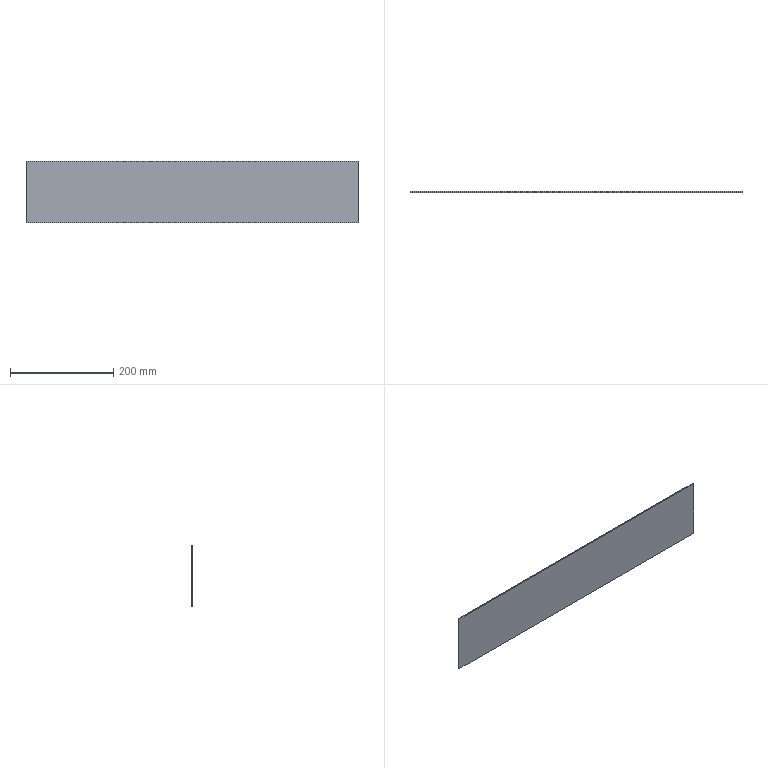Part | SolidWorks | features Extrusion 1 | 1 solid | 6 faces | box 642 x 2 x 118 mm | volume 151512 mm3 | plane 6
STEP:
#1=CARTESIAN_POINT('',(321.,0.,59.));
#2=VERTEX_POINT('',#1);
#3=CARTESIAN_POINT('',(321.,0.,-59.));
#4=VERTEX_POINT('',#3);
#5=CARTESIAN_POINT('',(321.,0.,-59.));
#6=DIRECTION('',(0.,0.,-1.));
#7=VECTOR('',#6,1000.);
#8=LINE('',#5,#7);
#9=EDGE_CURVE('',#2,#4,#8,.T.);
#10=ORIENTED_EDGE('',*,*,#9,.T.);
#11=CARTESIAN_POINT('',(321.,2.,-59.));
#12=VERTEX_POINT('',#11);
#13=CARTESIAN_POINT('',(321.,2.,-59.));
#14=DIRECTION('',(0.,-1.,0.));
#15=VECTOR('',#14,1000.);
#16=LINE('',#13,#15);
#17=EDGE_CURVE('',#12,#4,#16,.T.);
#18=ORIENTED_EDGE('',*,*,#17,.F.);
#19=CARTESIAN_POINT('',(321.,2.,59.));
#20=VERTEX_POINT('',#19);
#21=CARTESIAN_POINT('',(321.,2.,-59.));
#22=DIRECTION('',(0.,0.,-1.));
#23=VECTOR('',#22,1000.);
#24=LINE('',#21,#23);
#25=EDGE_CURVE('',#20,#12,#24,.T.);
#26=ORIENTED_EDGE('',*,*,#25,.F.);
#27=CARTESIAN_POINT('',(321.,2.,59.));
#28=DIRECTION('',(0.,-1.,0.));
#29=VECTOR('',#28,1000.);
#30=LINE('',#27,#29);
#31=EDGE_CURVE('',#20,#2,#30,.T.);
#32=ORIENTED_EDGE('',*,*,#31,.T.);
#33=EDGE_LOOP('',(#10,#18,#26,#32));
#34=FACE_OUTER_BOUND('',#33,.T.);
#35=CARTESIAN_POINT('',(321.,2.,-59.));
#36=DIRECTION('',(-1.,0.,0.));
#37=DIRECTION('',(0.,0.,1.));
#38=AXIS2_PLACEMENT_3D('',#35,#36,#37);
#39=PLANE('',#38);
#40=ADVANCED_FACE('',(#34),#39,.F.);
#41=CARTESIAN_POINT('',(-321.,0.,-59.));
#42=VERTEX_POINT('',#41);
#43=CARTESIAN_POINT('',(-321.,0.,-59.));
#44=DIRECTION('',(-1.,0.,0.));
#45=VECTOR('',#44,1000.);
#46=LINE('',#43,#45);
#47=EDGE_CURVE('',#4,#42,#46,.T.);
#48=ORIENTED_EDGE('',*,*,#47,.T.);
#49=CARTESIAN_POINT('',(-321.,2.,-59.));
#50=VERTEX_POINT('',#49);
#51=CARTESIAN_POINT('',(-321.,2.,-59.));
#52=DIRECTION('',(0.,-1.,0.));
#53=VECTOR('',#52,1000.);
#54=LINE('',#51,#53);
#55=EDGE_CURVE('',#50,#42,#54,.T.);
#56=ORIENTED_EDGE('',*,*,#55,.F.);
#57=CARTESIAN_POINT('',(-321.,2.,-59.));
#58=DIRECTION('',(-1.,0.,0.));
#59=VECTOR('',#58,1000.);
#60=LINE('',#57,#59);
#61=EDGE_CURVE('',#12,#50,#60,.T.);
#62=ORIENTED_EDGE('',*,*,#61,.F.);
#63=ORIENTED_EDGE('',*,*,#17,.T.);
#64=EDGE_LOOP('',(#48,#56,#62,#63));
#65=FACE_OUTER_BOUND('',#64,.T.);
#66=CARTESIAN_POINT('',(-321.,2.,-59.));
#67=DIRECTION('',(0.,0.,1.));
#68=DIRECTION('',(1.,0.,0.));
#69=AXIS2_PLACEMENT_3D('',#66,#67,#68);
#70=PLANE('',#69);
#71=ADVANCED_FACE('',(#65),#70,.F.);
#72=CARTESIAN_POINT('',(-321.,0.,59.));
#73=VERTEX_POINT('',#72);
#74=CARTESIAN_POINT('',(-321.,0.,-59.));
#75=DIRECTION('',(0.,0.,1.));
#76=VECTOR('',#75,1000.);
#77=LINE('',#74,#76);
#78=EDGE_CURVE('',#42,#73,#77,.T.);
#79=ORIENTED_EDGE('',*,*,#78,.T.);
#80=CARTESIAN_POINT('',(-321.,2.,59.));
#81=VERTEX_POINT('',#80);
#82=CARTESIAN_POINT('',(-321.,2.,59.));
#83=DIRECTION('',(0.,-1.,0.));
#84=VECTOR('',#83,1000.);
#85=LINE('',#82,#84);
#86=EDGE_CURVE('',#81,#73,#85,.T.);
#87=ORIENTED_EDGE('',*,*,#86,.F.);
#88=CARTESIAN_POINT('',(-321.,2.,-59.));
#89=DIRECTION('',(0.,0.,1.));
#90=VECTOR('',#89,1000.);
#91=LINE('',#88,#90);
#92=EDGE_CURVE('',#50,#81,#91,.T.);
#93=ORIENTED_EDGE('',*,*,#92,.F.);
#94=ORIENTED_EDGE('',*,*,#55,.T.);
#95=EDGE_LOOP('',(#79,#87,#93,#94));
#96=FACE_OUTER_BOUND('',#95,.T.);
#97=CARTESIAN_POINT('',(-321.,2.,-59.));
#98=DIRECTION('',(1.,0.,0.));
#99=DIRECTION('',(0.,0.,-1.));
#100=AXIS2_PLACEMENT_3D('',#97,#98,#99);
#101=PLANE('',#100);
#102=ADVANCED_FACE('',(#96),#101,.F.);
#103=CARTESIAN_POINT('',(-321.,0.,59.));
#104=DIRECTION('',(1.,0.,0.));
#105=VECTOR('',#104,1000.);
#106=LINE('',#103,#105);
#107=EDGE_CURVE('',#73,#2,#106,.T.);
#108=ORIENTED_EDGE('',*,*,#107,.T.);
#109=ORIENTED_EDGE('',*,*,#31,.F.);
#110=CARTESIAN_POINT('',(-321.,2.,59.));
#111=DIRECTION('',(1.,0.,0.));
#112=VECTOR('',#111,1000.);
#113=LINE('',#110,#112);
#114=EDGE_CURVE('',#81,#20,#113,.T.);
#115=ORIENTED_EDGE('',*,*,#114,.F.);
#116=ORIENTED_EDGE('',*,*,#86,.T.);
#117=EDGE_LOOP('',(#108,#109,#115,#116));
#118=FACE_OUTER_BOUND('',#117,.T.);
#119=CARTESIAN_POINT('',(-321.,2.,59.));
#120=DIRECTION('',(0.,0.,-1.));
#121=DIRECTION('',(-1.,0.,0.));
#122=AXIS2_PLACEMENT_3D('',#119,#120,#121);
#123=PLANE('',#122);
#124=ADVANCED_FACE('',(#118),#123,.F.);
#125=ORIENTED_EDGE('',*,*,#25,.T.);
#126=ORIENTED_EDGE('',*,*,#61,.T.);
#127=ORIENTED_EDGE('',*,*,#92,.T.);
#128=ORIENTED_EDGE('',*,*,#114,.T.);
#129=EDGE_LOOP('',(#125,#126,#127,#128));
#130=FACE_OUTER_BOUND('',#129,.T.);
#131=CARTESIAN_POINT('',(0.,2.,0.));
#132=DIRECTION('',(0.,1.,0.));
#133=DIRECTION('',(0.,0.,1.));
#134=AXIS2_PLACEMENT_3D('',#131,#132,#133);
#135=PLANE('',#134);
#136=ADVANCED_FACE('',(#130),#135,.T.);
#137=ORIENTED_EDGE('',*,*,#9,.F.);
#138=ORIENTED_EDGE('',*,*,#107,.F.);
#139=ORIENTED_EDGE('',*,*,#78,.F.);
#140=ORIENTED_EDGE('',*,*,#47,.F.);
#141=EDGE_LOOP('',(#137,#138,#139,#140));
#142=FACE_OUTER_BOUND('',#141,.T.);
#143=CARTESIAN_POINT('',(0.,0.,0.));
#144=DIRECTION('',(0.,1.,0.));
#145=DIRECTION('',(0.,0.,1.));
#146=AXIS2_PLACEMENT_3D('',#143,#144,#145);
#147=PLANE('',#146);
#148=ADVANCED_FACE('',(#142),#147,.F.);
#149=CLOSED_SHELL('',(#40,#71,#102,#124,#136,#148));
#150=MANIFOLD_SOLID_BREP('',#149);
#151=CARTESIAN_POINT('',(0.,0.,0.));
#152=DIRECTION('',(0.,0.,1.));
#153=DIRECTION('',(1.,0.,0.));
#154=AXIS2_PLACEMENT_3D('',#151,#152,#153);
#155=(LENGTH_UNIT()NAMED_UNIT(*)SI_UNIT(.MILLI.,.METRE.));
#156=UNCERTAINTY_MEASURE_WITH_UNIT(LENGTH_MEASURE(0.00001),#155,'','');
#157=(NAMED_UNIT(*)PLANE_ANGLE_UNIT()SI_UNIT($,.RADIAN.));
#158=(NAMED_UNIT(*)SI_UNIT($,.STERADIAN.)SOLID_ANGLE_UNIT());
#159=(GEOMETRIC_REPRESENTATION_CONTEXT(3)GLOBAL_UNCERTAINTY_ASSIGNED_CONTEXT((#156))GLOBAL_UNIT_ASSIGNED_CONTEXT((#155,#157,#158))REPRESENTATION_CONTEXT('',''));
#160=ADVANCED_BREP_SHAPE_REPRESENTATION('',(#150,#154),#159);